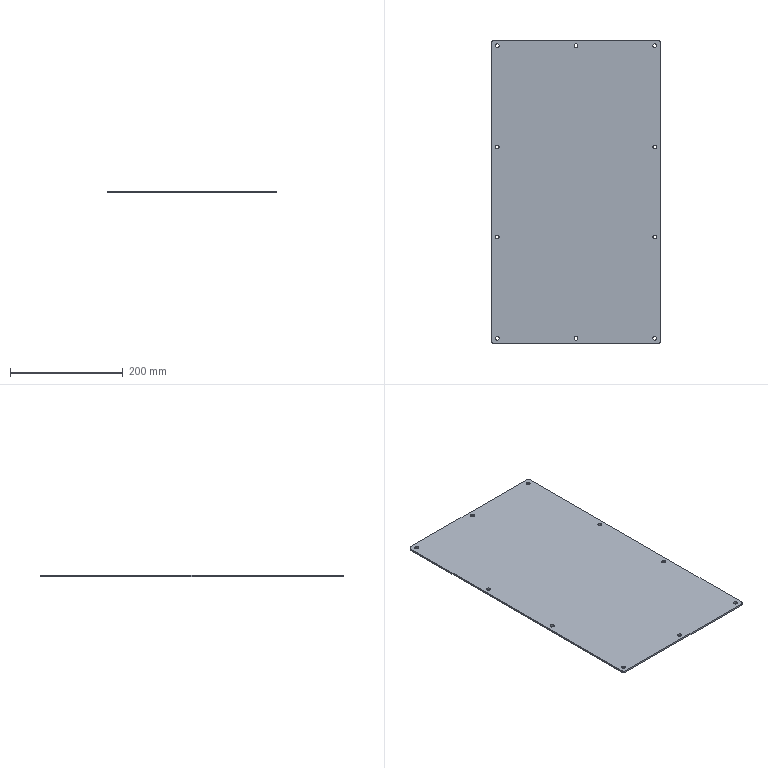Part | SolidWorks | features BaseBody 1 | 1 solid | 30 faces | box 300 x 540 x 3 mm | volume 484781 mm3 | cylinder 24 | plane 6 | commonest cylinder face diameters 7 x20 10 x4
STEP:
#1=CARTESIAN_POINT('',(136.5,-260.,0.));
#2=VERTEX_POINT('',#1);
#3=CARTESIAN_POINT('',(143.5,-260.,0.));
#4=VERTEX_POINT('',#3);
#5=CARTESIAN_POINT('',(140.,-260.,0.));
#6=DIRECTION('',(0.,0.,1.));
#7=DIRECTION('',(1.,0.,0.));
#8=AXIS2_PLACEMENT_3D('',#5,#6,#7);
#9=CIRCLE('',#8,3.5);
#10=EDGE_CURVE('',#2,#4,#9,.T.);
#11=ORIENTED_EDGE('',*,*,#10,.F.);
#12=CARTESIAN_POINT('',(136.5,-260.,3.));
#13=VERTEX_POINT('',#12);
#14=CARTESIAN_POINT('',(136.5,-260.,3.));
#15=DIRECTION('',(0.,0.,1.));
#16=VECTOR('',#15,1000.);
#17=LINE('',#14,#16);
#18=EDGE_CURVE('',#2,#13,#17,.T.);
#19=ORIENTED_EDGE('',*,*,#18,.T.);
#20=CARTESIAN_POINT('',(143.5,-260.,3.));
#21=VERTEX_POINT('',#20);
#22=CARTESIAN_POINT('',(140.,-260.,3.));
#23=DIRECTION('',(0.,0.,1.));
#24=DIRECTION('',(1.,0.,0.));
#25=AXIS2_PLACEMENT_3D('',#22,#23,#24);
#26=CIRCLE('',#25,3.5);
#27=EDGE_CURVE('',#13,#21,#26,.T.);
#28=ORIENTED_EDGE('',*,*,#27,.T.);
#29=CARTESIAN_POINT('',(143.5,-260.,3.));
#30=DIRECTION('',(0.,0.,1.));
#31=VECTOR('',#30,1000.);
#32=LINE('',#29,#31);
#33=EDGE_CURVE('',#4,#21,#32,.T.);
#34=ORIENTED_EDGE('',*,*,#33,.F.);
#35=EDGE_LOOP('',(#11,#19,#28,#34));
#36=FACE_OUTER_BOUND('',#35,.T.);
#37=CARTESIAN_POINT('',(140.,-260.,3.));
#38=DIRECTION('',(0.,0.,1.));
#39=DIRECTION('',(1.,0.,0.));
#40=AXIS2_PLACEMENT_3D('',#37,#38,#39);
#41=CYLINDRICAL_SURFACE('',#40,3.5);
#42=ADVANCED_FACE('',(#36),#41,.F.);
#43=CARTESIAN_POINT('',(-143.5,260.,0.));
#44=VERTEX_POINT('',#43);
#45=CARTESIAN_POINT('',(-136.5,260.,0.));
#46=VERTEX_POINT('',#45);
#47=CARTESIAN_POINT('',(-140.,260.,0.));
#48=DIRECTION('',(0.,0.,1.));
#49=DIRECTION('',(1.,0.,0.));
#50=AXIS2_PLACEMENT_3D('',#47,#48,#49);
#51=CIRCLE('',#50,3.5);
#52=EDGE_CURVE('',#44,#46,#51,.T.);
#53=ORIENTED_EDGE('',*,*,#52,.F.);
#54=CARTESIAN_POINT('',(-143.5,260.,3.));
#55=VERTEX_POINT('',#54);
#56=CARTESIAN_POINT('',(-143.5,260.,3.));
#57=DIRECTION('',(0.,0.,1.));
#58=VECTOR('',#57,1000.);
#59=LINE('',#56,#58);
#60=EDGE_CURVE('',#44,#55,#59,.T.);
#61=ORIENTED_EDGE('',*,*,#60,.T.);
#62=CARTESIAN_POINT('',(-136.5,260.,3.));
#63=VERTEX_POINT('',#62);
#64=CARTESIAN_POINT('',(-140.,260.,3.));
#65=DIRECTION('',(0.,0.,1.));
#66=DIRECTION('',(1.,0.,0.));
#67=AXIS2_PLACEMENT_3D('',#64,#65,#66);
#68=CIRCLE('',#67,3.5);
#69=EDGE_CURVE('',#55,#63,#68,.T.);
#70=ORIENTED_EDGE('',*,*,#69,.T.);
#71=CARTESIAN_POINT('',(-136.5,260.,3.));
#72=DIRECTION('',(0.,0.,1.));
#73=VECTOR('',#72,1000.);
#74=LINE('',#71,#73);
#75=EDGE_CURVE('',#46,#63,#74,.T.);
#76=ORIENTED_EDGE('',*,*,#75,.F.);
#77=EDGE_LOOP('',(#53,#61,#70,#76));
#78=FACE_OUTER_BOUND('',#77,.T.);
#79=CARTESIAN_POINT('',(-140.,260.,3.));
#80=DIRECTION('',(0.,0.,1.));
#81=DIRECTION('',(1.,0.,0.));
#82=AXIS2_PLACEMENT_3D('',#79,#80,#81);
#83=CYLINDRICAL_SURFACE('',#82,3.5);
#84=ADVANCED_FACE('',(#78),#83,.F.);
#85=CARTESIAN_POINT('',(-143.5,-260.,0.));
#86=VERTEX_POINT('',#85);
#87=CARTESIAN_POINT('',(-136.5,-260.,0.));
#88=VERTEX_POINT('',#87);
#89=CARTESIAN_POINT('',(-140.,-260.,0.));
#90=DIRECTION('',(0.,0.,1.));
#91=DIRECTION('',(1.,0.,0.));
#92=AXIS2_PLACEMENT_3D('',#89,#90,#91);
#93=CIRCLE('',#92,3.5);
#94=EDGE_CURVE('',#86,#88,#93,.T.);
#95=ORIENTED_EDGE('',*,*,#94,.F.);
#96=CARTESIAN_POINT('',(-143.5,-260.,3.));
#97=VERTEX_POINT('',#96);
#98=CARTESIAN_POINT('',(-143.5,-260.,3.));
#99=DIRECTION('',(0.,0.,1.));
#100=VECTOR('',#99,1000.);
#101=LINE('',#98,#100);
#102=EDGE_CURVE('',#86,#97,#101,.T.);
#103=ORIENTED_EDGE('',*,*,#102,.T.);
#104=CARTESIAN_POINT('',(-136.5,-260.,3.));
#105=VERTEX_POINT('',#104);
#106=CARTESIAN_POINT('',(-140.,-260.,3.));
#107=DIRECTION('',(0.,0.,1.));
#108=DIRECTION('',(1.,0.,0.));
#109=AXIS2_PLACEMENT_3D('',#106,#107,#108);
#110=CIRCLE('',#109,3.5);
#111=EDGE_CURVE('',#97,#105,#110,.T.);
#112=ORIENTED_EDGE('',*,*,#111,.T.);
#113=CARTESIAN_POINT('',(-136.5,-260.,3.));
#114=DIRECTION('',(0.,0.,1.));
#115=VECTOR('',#114,1000.);
#116=LINE('',#113,#115);
#117=EDGE_CURVE('',#88,#105,#116,.T.);
#118=ORIENTED_EDGE('',*,*,#117,.F.);
#119=EDGE_LOOP('',(#95,#103,#112,#118));
#120=FACE_OUTER_BOUND('',#119,.T.);
#121=CARTESIAN_POINT('',(-140.,-260.,3.));
#122=DIRECTION('',(0.,0.,1.));
#123=DIRECTION('',(1.,0.,0.));
#124=AXIS2_PLACEMENT_3D('',#121,#122,#123);
#125=CYLINDRICAL_SURFACE('',#124,3.5);
#126=ADVANCED_FACE('',(#120),#125,.F.);
#127=CARTESIAN_POINT('',(136.5,260.,0.));
#128=VERTEX_POINT('',#127);
#129=CARTESIAN_POINT('',(143.5,260.,0.));
#130=VERTEX_POINT('',#129);
#131=CARTESIAN_POINT('',(140.,260.,0.));
#132=DIRECTION('',(0.,0.,1.));
#133=DIRECTION('',(1.,0.,0.));
#134=AXIS2_PLACEMENT_3D('',#131,#132,#133);
#135=CIRCLE('',#134,3.5);
#136=EDGE_CURVE('',#128,#130,#135,.T.);
#137=ORIENTED_EDGE('',*,*,#136,.F.);
#138=CARTESIAN_POINT('',(136.5,260.,3.));
#139=VERTEX_POINT('',#138);
#140=CARTESIAN_POINT('',(136.5,260.,3.));
#141=DIRECTION('',(0.,0.,1.));
#142=VECTOR('',#141,1000.);
#143=LINE('',#140,#142);
#144=EDGE_CURVE('',#128,#139,#143,.T.);
#145=ORIENTED_EDGE('',*,*,#144,.T.);
#146=CARTESIAN_POINT('',(143.5,260.,3.));
#147=VERTEX_POINT('',#146);
#148=CARTESIAN_POINT('',(140.,260.,3.));
#149=DIRECTION('',(0.,0.,1.));
#150=DIRECTION('',(1.,0.,0.));
#151=AXIS2_PLACEMENT_3D('',#148,#149,#150);
#152=CIRCLE('',#151,3.5);
#153=EDGE_CURVE('',#139,#147,#152,.T.);
#154=ORIENTED_EDGE('',*,*,#153,.T.);
#155=CARTESIAN_POINT('',(143.5,260.,3.));
#156=DIRECTION('',(0.,0.,1.));
#157=VECTOR('',#156,1000.);
#158=LINE('',#155,#157);
#159=EDGE_CURVE('',#130,#147,#158,.T.);
#160=ORIENTED_EDGE('',*,*,#159,.F.);
#161=EDGE_LOOP('',(#137,#145,#154,#160));
#162=FACE_OUTER_BOUND('',#161,.T.);
#163=CARTESIAN_POINT('',(140.,260.,3.));
#164=DIRECTION('',(0.,0.,1.));
#165=DIRECTION('',(1.,0.,0.));
#166=AXIS2_PLACEMENT_3D('',#163,#164,#165);
#167=CYLINDRICAL_SURFACE('',#166,3.5);
#168=ADVANCED_FACE('',(#162),#167,.F.);
#169=CARTESIAN_POINT('',(-3.5,260.,0.));
#170=VERTEX_POINT('',#169);
#171=CARTESIAN_POINT('',(3.5,260.,0.));
#172=VERTEX_POINT('',#171);
#173=CARTESIAN_POINT('',(0.,260.,0.));
#174=DIRECTION('',(0.,0.,1.));
#175=DIRECTION('',(1.,0.,0.));
#176=AXIS2_PLACEMENT_3D('',#173,#174,#175);
#177=CIRCLE('',#176,3.5);
#178=EDGE_CURVE('',#170,#172,#177,.T.);
#179=ORIENTED_EDGE('',*,*,#178,.F.);
#180=CARTESIAN_POINT('',(-3.5,260.,3.));
#181=VERTEX_POINT('',#180);
#182=CARTESIAN_POINT('',(-3.5,260.,3.));
#183=DIRECTION('',(0.,0.,1.));
#184=VECTOR('',#183,1000.);
#185=LINE('',#182,#184);
#186=EDGE_CURVE('',#170,#181,#185,.T.);
#187=ORIENTED_EDGE('',*,*,#186,.T.);
#188=CARTESIAN_POINT('',(3.5,260.,3.));
#189=VERTEX_POINT('',#188);
#190=CARTESIAN_POINT('',(0.,260.,3.));
#191=DIRECTION('',(0.,0.,1.));
#192=DIRECTION('',(1.,0.,0.));
#193=AXIS2_PLACEMENT_3D('',#190,#191,#192);
#194=CIRCLE('',#193,3.5);
#195=EDGE_CURVE('',#181,#189,#194,.T.);
#196=ORIENTED_EDGE('',*,*,#195,.T.);
#197=CARTESIAN_POINT('',(3.5,260.,3.));
#198=DIRECTION('',(0.,0.,1.));
#199=VECTOR('',#198,1000.);
#200=LINE('',#197,#199);
#201=EDGE_CURVE('',#172,#189,#200,.T.);
#202=ORIENTED_EDGE('',*,*,#201,.F.);
#203=EDGE_LOOP('',(#179,#187,#196,#202));
#204=FACE_OUTER_BOUND('',#203,.T.);
#205=CARTESIAN_POINT('',(0.,260.,3.));
#206=DIRECTION('',(0.,0.,1.));
#207=DIRECTION('',(1.,0.,0.));
#208=AXIS2_PLACEMENT_3D('',#205,#206,#207);
#209=CYLINDRICAL_SURFACE('',#208,3.5);
#210=ADVANCED_FACE('',(#204),#209,.F.);
#211=CARTESIAN_POINT('',(-3.5,-260.,0.));
#212=VERTEX_POINT('',#211);
#213=CARTESIAN_POINT('',(3.5,-260.,0.));
#214=VERTEX_POINT('',#213);
#215=CARTESIAN_POINT('',(0.,-260.,0.));
#216=DIRECTION('',(0.,0.,1.));
#217=DIRECTION('',(1.,0.,0.));
#218=AXIS2_PLACEMENT_3D('',#215,#216,#217);
#219=CIRCLE('',#218,3.5);
#220=EDGE_CURVE('',#212,#214,#219,.T.);
#221=ORIENTED_EDGE('',*,*,#220,.F.);
#222=CARTESIAN_POINT('',(-3.5,-260.,3.));
#223=VERTEX_POINT('',#222);
#224=CARTESIAN_POINT('',(-3.5,-260.,3.));
#225=DIRECTION('',(0.,0.,1.));
#226=VECTOR('',#225,1000.);
#227=LINE('',#224,#226);
#228=EDGE_CURVE('',#212,#223,#227,.T.);
#229=ORIENTED_EDGE('',*,*,#228,.T.);
#230=CARTESIAN_POINT('',(3.5,-260.,3.));
#231=VERTEX_POINT('',#230);
#232=CARTESIAN_POINT('',(0.,-260.,3.));
#233=DIRECTION('',(0.,0.,1.));
#234=DIRECTION('',(1.,0.,0.));
#235=AXIS2_PLACEMENT_3D('',#232,#233,#234);
#236=CIRCLE('',#235,3.5);
#237=EDGE_CURVE('',#223,#231,#236,.T.);
#238=ORIENTED_EDGE('',*,*,#237,.T.);
#239=CARTESIAN_POINT('',(3.5,-260.,3.));
#240=DIRECTION('',(0.,0.,1.));
#241=VECTOR('',#240,1000.);
#242=LINE('',#239,#241);
#243=EDGE_CURVE('',#214,#231,#242,.T.);
#244=ORIENTED_EDGE('',*,*,#243,.F.);
#245=EDGE_LOOP('',(#221,#229,#238,#244));
#246=FACE_OUTER_BOUND('',#245,.T.);
#247=CARTESIAN_POINT('',(0.,-260.,3.));
#248=DIRECTION('',(0.,0.,1.));
#249=DIRECTION('',(1.,0.,0.));
#250=AXIS2_PLACEMENT_3D('',#247,#248,#249);
#251=CYLINDRICAL_SURFACE('',#250,3.5);
#252=ADVANCED_FACE('',(#246),#251,.F.);
#253=CARTESIAN_POINT('',(-143.5,-80.,0.));
#254=VERTEX_POINT('',#253);
#255=CARTESIAN_POINT('',(-136.5,-80.,0.));
#256=VERTEX_POINT('',#255);
#257=CARTESIAN_POINT('',(-140.,-80.,0.));
#258=DIRECTION('',(0.,0.,1.));
#259=DIRECTION('',(1.,0.,0.));
#260=AXIS2_PLACEMENT_3D('',#257,#258,#259);
#261=CIRCLE('',#260,3.5);
#262=EDGE_CURVE('',#254,#256,#261,.T.);
#263=ORIENTED_EDGE('',*,*,#262,.F.);
#264=CARTESIAN_POINT('',(-143.5,-80.,3.));
#265=VERTEX_POINT('',#264);
#266=CARTESIAN_POINT('',(-143.5,-80.,3.));
#267=DIRECTION('',(0.,0.,1.));
#268=VECTOR('',#267,1000.);
#269=LINE('',#266,#268);
#270=EDGE_CURVE('',#254,#265,#269,.T.);
#271=ORIENTED_EDGE('',*,*,#270,.T.);
#272=CARTESIAN_POINT('',(-136.5,-80.,3.));
#273=VERTEX_POINT('',#272);
#274=CARTESIAN_POINT('',(-140.,-80.,3.));
#275=DIRECTION('',(0.,0.,1.));
#276=DIRECTION('',(1.,0.,0.));
#277=AXIS2_PLACEMENT_3D('',#274,#275,#276);
#278=CIRCLE('',#277,3.5);
#279=EDGE_CURVE('',#265,#273,#278,.T.);
#280=ORIENTED_EDGE('',*,*,#279,.T.);
#281=CARTESIAN_POINT('',(-136.5,-80.,3.));
#282=DIRECTION('',(0.,0.,1.));
#283=VECTOR('',#282,1000.);
#284=LINE('',#281,#283);
#285=EDGE_CURVE('',#256,#273,#284,.T.);
#286=ORIENTED_EDGE('',*,*,#285,.F.);
#287=EDGE_LOOP('',(#263,#271,#280,#286));
#288=FACE_OUTER_BOUND('',#287,.T.);
#289=CARTESIAN_POINT('',(-140.,-80.,3.));
#290=DIRECTION('',(0.,0.,1.));
#291=DIRECTION('',(1.,0.,0.));
#292=AXIS2_PLACEMENT_3D('',#289,#290,#291);
#293=CYLINDRICAL_SURFACE('',#292,3.5);
#294=ADVANCED_FACE('',(#288),#293,.F.);
#295=CARTESIAN_POINT('',(-143.5,80.,0.));
#296=VERTEX_POINT('',#295);
#297=CARTESIAN_POINT('',(-136.5,80.,0.));
#298=VERTEX_POINT('',#297);
#299=CARTESIAN_POINT('',(-140.,80.,0.));
#300=DIRECTION('',(0.,0.,1.));
#301=DIRECTION('',(1.,0.,0.));
#302=AXIS2_PLACEMENT_3D('',#299,#300,#301);
#303=CIRCLE('',#302,3.5);
#304=EDGE_CURVE('',#296,#298,#303,.T.);
#305=ORIENTED_EDGE('',*,*,#304,.F.);
#306=CARTESIAN_POINT('',(-143.5,80.,3.));
#307=VERTEX_POINT('',#306);
#308=CARTESIAN_POINT('',(-143.5,80.,3.));
#309=DIRECTION('',(0.,0.,1.));
#310=VECTOR('',#309,1000.);
#311=LINE('',#308,#310);
#312=EDGE_CURVE('',#296,#307,#311,.T.);
#313=ORIENTED_EDGE('',*,*,#312,.T.);
#314=CARTESIAN_POINT('',(-136.5,80.,3.));
#315=VERTEX_POINT('',#314);
#316=CARTESIAN_POINT('',(-140.,80.,3.));
#317=DIRECTION('',(0.,0.,1.));
#318=DIRECTION('',(1.,0.,0.));
#319=AXIS2_PLACEMENT_3D('',#316,#317,#318);
#320=CIRCLE('',#319,3.5);
#321=EDGE_CURVE('',#307,#315,#320,.T.);
#322=ORIENTED_EDGE('',*,*,#321,.T.);
#323=CARTESIAN_POINT('',(-136.5,80.,3.));
#324=DIRECTION('',(0.,0.,1.));
#325=VECTOR('',#324,1000.);
#326=LINE('',#323,#325);
#327=EDGE_CURVE('',#298,#315,#326,.T.);
#328=ORIENTED_EDGE('',*,*,#327,.F.);
#329=EDGE_LOOP('',(#305,#313,#322,#328));
#330=FACE_OUTER_BOUND('',#329,.T.);
#331=CARTESIAN_POINT('',(-140.,80.,3.));
#332=DIRECTION('',(0.,0.,1.));
#333=DIRECTION('',(1.,0.,0.));
#334=AXIS2_PLACEMENT_3D('',#331,#332,#333);
#335=CYLINDRICAL_SURFACE('',#334,3.5);
#336=ADVANCED_FACE('',(#330),#335,.F.);
#337=CARTESIAN_POINT('',(136.5,80.,0.));
#338=VERTEX_POINT('',#337);
#339=CARTESIAN_POINT('',(143.5,80.,0.));
#340=VERTEX_POINT('',#339);
#341=CARTESIAN_POINT('',(140.,80.,0.));
#342=DIRECTION('',(0.,0.,1.));
#343=DIRECTION('',(1.,0.,0.));
#344=AXIS2_PLACEMENT_3D('',#341,#342,#343);
#345=CIRCLE('',#344,3.5);
#346=EDGE_CURVE('',#338,#340,#345,.T.);
#347=ORIENTED_EDGE('',*,*,#346,.F.);
#348=CARTESIAN_POINT('',(136.5,80.,3.));
#349=VERTEX_POINT('',#348);
#350=CARTESIAN_POINT('',(136.5,80.,3.));
#351=DIRECTION('',(0.,0.,1.));
#352=VECTOR('',#351,1000.);
#353=LINE('',#350,#352);
#354=EDGE_CURVE('',#338,#349,#353,.T.);
#355=ORIENTED_EDGE('',*,*,#354,.T.);
#356=CARTESIAN_POINT('',(143.5,80.,3.));
#357=VERTEX_POINT('',#356);
#358=CARTESIAN_POINT('',(140.,80.,3.));
#359=DIRECTION('',(0.,0.,1.));
#360=DIRECTION('',(1.,0.,0.));
#361=AXIS2_PLACEMENT_3D('',#358,#359,#360);
#362=CIRCLE('',#361,3.5);
#363=EDGE_CURVE('',#349,#357,#362,.T.);
#364=ORIENTED_EDGE('',*,*,#363,.T.);
#365=CARTESIAN_POINT('',(143.5,80.,3.));
#366=DIRECTION('',(0.,0.,1.));
#367=VECTOR('',#366,1000.);
#368=LINE('',#365,#367);
#369=EDGE_CURVE('',#340,#357,#368,.T.);
#370=ORIENTED_EDGE('',*,*,#369,.F.);
#371=EDGE_LOOP('',(#347,#355,#364,#370));
#372=FACE_OUTER_BOUND('',#371,.T.);
#373=CARTESIAN_POINT('',(140.,80.,3.));
#374=DIRECTION('',(0.,0.,1.));
#375=DIRECTION('',(1.,0.,0.));
#376=AXIS2_PLACEMENT_3D('',#373,#374,#375);
#377=CYLINDRICAL_SURFACE('',#376,3.5);
#378=ADVANCED_FACE('',(#372),#377,.F.);
#379=CARTESIAN_POINT('',(136.5,-80.,0.));
#380=VERTEX_POINT('',#379);
#381=CARTESIAN_POINT('',(143.5,-80.,0.));
#382=VERTEX_POINT('',#381);
#383=CARTESIAN_POINT('',(140.,-80.,0.));
#384=DIRECTION('',(0.,0.,1.));
#385=DIRECTION('',(1.,0.,0.));
#386=AXIS2_PLACEMENT_3D('',#383,#384,#385);
#387=CIRCLE('',#386,3.5);
#388=EDGE_CURVE('',#380,#382,#387,.T.);
#389=ORIENTED_EDGE('',*,*,#388,.F.);
#390=CARTESIAN_POINT('',(136.5,-80.,3.));
#391=VERTEX_POINT('',#390);
#392=CARTESIAN_POINT('',(136.5,-80.,3.));
#393=DIRECTION('',(0.,0.,1.));
#394=VECTOR('',#393,1000.);
#395=LINE('',#392,#394);
#396=EDGE_CURVE('',#380,#391,#395,.T.);
#397=ORIENTED_EDGE('',*,*,#396,.T.);
#398=CARTESIAN_POINT('',(143.5,-80.,3.));
#399=VERTEX_POINT('',#398);
#400=CARTESIAN_POINT('',(140.,-80.,3.));
#401=DIRECTION('',(0.,0.,1.));
#402=DIRECTION('',(1.,0.,0.));
#403=AXIS2_PLACEMENT_3D('',#400,#401,#402);
#404=CIRCLE('',#403,3.5);
#405=EDGE_CURVE('',#391,#399,#404,.T.);
#406=ORIENTED_EDGE('',*,*,#405,.T.);
#407=CARTESIAN_POINT('',(143.5,-80.,3.));
#408=DIRECTION('',(0.,0.,1.));
#409=VECTOR('',#408,1000.);
#410=LINE('',#407,#409);
#411=EDGE_CURVE('',#382,#399,#410,.T.);
#412=ORIENTED_EDGE('',*,*,#411,.F.);
#413=EDGE_LOOP('',(#389,#397,#406,#412));
#414=FACE_OUTER_BOUND('',#413,.T.);
#415=CARTESIAN_POINT('',(140.,-80.,3.));
#416=DIRECTION('',(0.,0.,1.));
#417=DIRECTION('',(1.,0.,0.));
#418=AXIS2_PLACEMENT_3D('',#415,#416,#417);
#419=CYLINDRICAL_SURFACE('',#418,3.5);
#420=ADVANCED_FACE('',(#414),#419,.F.);
#421=CARTESIAN_POINT('',(-150.,-265.,0.));
#422=VERTEX_POINT('',#421);
#423=CARTESIAN_POINT('',(-145.,-270.,0.));
#424=VERTEX_POINT('',#423);
#425=CARTESIAN_POINT('',(-145.,-265.,0.));
#426=DIRECTION('',(0.,0.,1.));
#427=DIRECTION('',(1.,0.,0.));
#428=AXIS2_PLACEMENT_3D('',#425,#426,#427);
#429=CIRCLE('',#428,5.);
#430=EDGE_CURVE('',#422,#424,#429,.T.);
#431=ORIENTED_EDGE('',*,*,#430,.T.);
#432=CARTESIAN_POINT('',(-145.,-270.,3.));
#433=VERTEX_POINT('',#432);
#434=CARTESIAN_POINT('',(-145.,-270.,3.));
#435=DIRECTION('',(0.,0.,-1.));
#436=VECTOR('',#435,1000.);
#437=LINE('',#434,#436);
#438=EDGE_CURVE('',#433,#424,#437,.T.);
#439=ORIENTED_EDGE('',*,*,#438,.F.);
#440=CARTESIAN_POINT('',(-150.,-265.,3.));
#441=VERTEX_POINT('',#440);
#442=CARTESIAN_POINT('',(-145.,-265.,3.));
#443=DIRECTION('',(0.,0.,1.));
#444=DIRECTION('',(1.,0.,0.));
#445=AXIS2_PLACEMENT_3D('',#442,#443,#444);
#446=CIRCLE('',#445,5.);
#447=EDGE_CURVE('',#441,#433,#446,.T.);
#448=ORIENTED_EDGE('',*,*,#447,.F.);
#449=CARTESIAN_POINT('',(-150.,-265.,3.));
#450=DIRECTION('',(0.,0.,-1.));
#451=VECTOR('',#450,1000.);
#452=LINE('',#449,#451);
#453=EDGE_CURVE('',#441,#422,#452,.T.);
#454=ORIENTED_EDGE('',*,*,#453,.T.);
#455=EDGE_LOOP('',(#431,#439,#448,#454));
#456=FACE_OUTER_BOUND('',#455,.T.);
#457=CARTESIAN_POINT('',(-145.,-265.,3.));
#458=DIRECTION('',(0.,0.,-1.));
#459=DIRECTION('',(-1.,0.,0.));
#460=AXIS2_PLACEMENT_3D('',#457,#458,#459);
#461=CYLINDRICAL_SURFACE('',#460,5.);
#462=ADVANCED_FACE('',(#456),#461,.T.);
#463=CARTESIAN_POINT('',(145.,-270.,0.));
#464=VERTEX_POINT('',#463);
#465=CARTESIAN_POINT('',(-145.,-270.,0.));
#466=DIRECTION('',(1.,0.,0.));
#467=VECTOR('',#466,1000.);
#468=LINE('',#465,#467);
#469=EDGE_CURVE('',#424,#464,#468,.T.);
#470=ORIENTED_EDGE('',*,*,#469,.T.);
#471=CARTESIAN_POINT('',(145.,-270.,3.));
#472=VERTEX_POINT('',#471);
#473=CARTESIAN_POINT('',(145.,-270.,3.));
#474=DIRECTION('',(0.,0.,-1.));
#475=VECTOR('',#474,1000.);
#476=LINE('',#473,#475);
#477=EDGE_CURVE('',#472,#464,#476,.T.);
#478=ORIENTED_EDGE('',*,*,#477,.F.);
#479=CARTESIAN_POINT('',(-145.,-270.,3.));
#480=DIRECTION('',(1.,0.,0.));
#481=VECTOR('',#480,1000.);
#482=LINE('',#479,#481);
#483=EDGE_CURVE('',#433,#472,#482,.T.);
#484=ORIENTED_EDGE('',*,*,#483,.F.);
#485=ORIENTED_EDGE('',*,*,#438,.T.);
#486=EDGE_LOOP('',(#470,#478,#484,#485));
#487=FACE_OUTER_BOUND('',#486,.T.);
#488=CARTESIAN_POINT('',(-145.,-270.,3.));
#489=DIRECTION('',(0.,1.,0.));
#490=DIRECTION('',(0.,0.,1.));
#491=AXIS2_PLACEMENT_3D('',#488,#489,#490);
#492=PLANE('',#491);
#493=ADVANCED_FACE('',(#487),#492,.F.);
#494=CARTESIAN_POINT('',(150.,-265.,0.));
#495=VERTEX_POINT('',#494);
#496=CARTESIAN_POINT('',(145.,-265.,0.));
#497=DIRECTION('',(0.,0.,1.));
#498=DIRECTION('',(1.,0.,0.));
#499=AXIS2_PLACEMENT_3D('',#496,#497,#498);
#500=CIRCLE('',#499,5.);
#501=EDGE_CURVE('',#464,#495,#500,.T.);
#502=ORIENTED_EDGE('',*,*,#501,.T.);
#503=CARTESIAN_POINT('',(150.,-265.,3.));
#504=VERTEX_POINT('',#503);
#505=CARTESIAN_POINT('',(150.,-265.,3.));
#506=DIRECTION('',(0.,0.,-1.));
#507=VECTOR('',#506,1000.);
#508=LINE('',#505,#507);
#509=EDGE_CURVE('',#504,#495,#508,.T.);
#510=ORIENTED_EDGE('',*,*,#509,.F.);
#511=CARTESIAN_POINT('',(145.,-265.,3.));
#512=DIRECTION('',(0.,0.,1.));
#513=DIRECTION('',(1.,0.,0.));
#514=AXIS2_PLACEMENT_3D('',#511,#512,#513);
#515=CIRCLE('',#514,5.);
#516=EDGE_CURVE('',#472,#504,#515,.T.);
#517=ORIENTED_EDGE('',*,*,#516,.F.);
#518=ORIENTED_EDGE('',*,*,#477,.T.);
#519=EDGE_LOOP('',(#502,#510,#517,#518));
#520=FACE_OUTER_BOUND('',#519,.T.);
#521=CARTESIAN_POINT('',(145.,-265.,3.));
#522=DIRECTION('',(0.,0.,-1.));
#523=DIRECTION('',(-1.,0.,0.));
#524=AXIS2_PLACEMENT_3D('',#521,#522,#523);
#525=CYLINDRICAL_SURFACE('',#524,5.);
#526=ADVANCED_FACE('',(#520),#525,.T.);
#527=CARTESIAN_POINT('',(150.,265.,0.));
#528=VERTEX_POINT('',#527);
#529=CARTESIAN_POINT('',(150.,265.,0.));
#530=DIRECTION('',(0.,1.,0.));
#531=VECTOR('',#530,1000.);
#532=LINE('',#529,#531);
#533=EDGE_CURVE('',#495,#528,#532,.T.);
#534=ORIENTED_EDGE('',*,*,#533,.T.);
#535=CARTESIAN_POINT('',(150.,265.,3.));
#536=VERTEX_POINT('',#535);
#537=CARTESIAN_POINT('',(150.,265.,3.));
#538=DIRECTION('',(0.,0.,-1.));
#539=VECTOR('',#538,1000.);
#540=LINE('',#537,#539);
#541=EDGE_CURVE('',#536,#528,#540,.T.);
#542=ORIENTED_EDGE('',*,*,#541,.F.);
#543=CARTESIAN_POINT('',(150.,265.,3.));
#544=DIRECTION('',(0.,1.,0.));
#545=VECTOR('',#544,1000.);
#546=LINE('',#543,#545);
#547=EDGE_CURVE('',#504,#536,#546,.T.);
#548=ORIENTED_EDGE('',*,*,#547,.F.);
#549=ORIENTED_EDGE('',*,*,#509,.T.);
#550=EDGE_LOOP('',(#534,#542,#548,#549));
#551=FACE_OUTER_BOUND('',#550,.T.);
#552=CARTESIAN_POINT('',(150.,265.,3.));
#553=DIRECTION('',(-1.,0.,0.));
#554=DIRECTION('',(0.,-1.,0.));
#555=AXIS2_PLACEMENT_3D('',#552,#553,#554);
#556=PLANE('',#555);
#557=ADVANCED_FACE('',(#551),#556,.F.);
#558=CARTESIAN_POINT('',(145.,270.,0.));
#559=VERTEX_POINT('',#558);
#560=CARTESIAN_POINT('',(145.,265.,0.));
#561=DIRECTION('',(0.,0.,1.));
#562=DIRECTION('',(-1.,0.,0.));
#563=AXIS2_PLACEMENT_3D('',#560,#561,#562);
#564=CIRCLE('',#563,5.);
#565=EDGE_CURVE('',#528,#559,#564,.T.);
#566=ORIENTED_EDGE('',*,*,#565,.T.);
#567=CARTESIAN_POINT('',(145.,270.,3.));
#568=VERTEX_POINT('',#567);
#569=CARTESIAN_POINT('',(145.,270.,3.));
#570=DIRECTION('',(0.,0.,-1.));
#571=VECTOR('',#570,1000.);
#572=LINE('',#569,#571);
#573=EDGE_CURVE('',#568,#559,#572,.T.);
#574=ORIENTED_EDGE('',*,*,#573,.F.);
#575=CARTESIAN_POINT('',(145.,265.,3.));
#576=DIRECTION('',(0.,0.,1.));
#577=DIRECTION('',(-1.,0.,0.));
#578=AXIS2_PLACEMENT_3D('',#575,#576,#577);
#579=CIRCLE('',#578,5.);
#580=EDGE_CURVE('',#536,#568,#579,.T.);
#581=ORIENTED_EDGE('',*,*,#580,.F.);
#582=ORIENTED_EDGE('',*,*,#541,.T.);
#583=EDGE_LOOP('',(#566,#574,#581,#582));
#584=FACE_OUTER_BOUND('',#583,.T.);
#585=CARTESIAN_POINT('',(145.,265.,3.));
#586=DIRECTION('',(0.,0.,-1.));
#587=DIRECTION('',(-1.,0.,0.));
#588=AXIS2_PLACEMENT_3D('',#585,#586,#587);
#589=CYLINDRICAL_SURFACE('',#588,5.);
#590=ADVANCED_FACE('',(#584),#589,.T.);
#591=CARTESIAN_POINT('',(-145.,270.,0.));
#592=VERTEX_POINT('',#591);
#593=CARTESIAN_POINT('',(-145.,270.,0.));
#594=DIRECTION('',(-1.,0.,0.));
#595=VECTOR('',#594,1000.);
#596=LINE('',#593,#595);
#597=EDGE_CURVE('',#559,#592,#596,.T.);
#598=ORIENTED_EDGE('',*,*,#597,.T.);
#599=CARTESIAN_POINT('',(-145.,270.,3.));
#600=VERTEX_POINT('',#599);
#601=CARTESIAN_POINT('',(-145.,270.,3.));
#602=DIRECTION('',(0.,0.,-1.));
#603=VECTOR('',#602,1000.);
#604=LINE('',#601,#603);
#605=EDGE_CURVE('',#600,#592,#604,.T.);
#606=ORIENTED_EDGE('',*,*,#605,.F.);
#607=CARTESIAN_POINT('',(-145.,270.,3.));
#608=DIRECTION('',(-1.,0.,0.));
#609=VECTOR('',#608,1000.);
#610=LINE('',#607,#609);
#611=EDGE_CURVE('',#568,#600,#610,.T.);
#612=ORIENTED_EDGE('',*,*,#611,.F.);
#613=ORIENTED_EDGE('',*,*,#573,.T.);
#614=EDGE_LOOP('',(#598,#606,#612,#613));
#615=FACE_OUTER_BOUND('',#614,.T.);
#616=CARTESIAN_POINT('',(-145.,270.,3.));
#617=DIRECTION('',(0.,-1.,0.));
#618=DIRECTION('',(0.,0.,-1.));
#619=AXIS2_PLACEMENT_3D('',#616,#617,#618);
#620=PLANE('',#619);
#621=ADVANCED_FACE('',(#615),#620,.F.);
#622=CARTESIAN_POINT('',(-150.,265.,0.));
#623=VERTEX_POINT('',#622);
#624=CARTESIAN_POINT('',(-145.,265.,0.));
#625=DIRECTION('',(0.,0.,1.));
#626=DIRECTION('',(1.,0.,0.));
#627=AXIS2_PLACEMENT_3D('',#624,#625,#626);
#628=CIRCLE('',#627,5.);
#629=EDGE_CURVE('',#592,#623,#628,.T.);
#630=ORIENTED_EDGE('',*,*,#629,.T.);
#631=CARTESIAN_POINT('',(-150.,265.,3.));
#632=VERTEX_POINT('',#631);
#633=CARTESIAN_POINT('',(-150.,265.,3.));
#634=DIRECTION('',(0.,0.,-1.));
#635=VECTOR('',#634,1000.);
#636=LINE('',#633,#635);
#637=EDGE_CURVE('',#632,#623,#636,.T.);
#638=ORIENTED_EDGE('',*,*,#637,.F.);
#639=CARTESIAN_POINT('',(-145.,265.,3.));
#640=DIRECTION('',(0.,0.,1.));
#641=DIRECTION('',(1.,0.,0.));
#642=AXIS2_PLACEMENT_3D('',#639,#640,#641);
#643=CIRCLE('',#642,5.);
#644=EDGE_CURVE('',#600,#632,#643,.T.);
#645=ORIENTED_EDGE('',*,*,#644,.F.);
#646=ORIENTED_EDGE('',*,*,#605,.T.);
#647=EDGE_LOOP('',(#630,#638,#645,#646));
#648=FACE_OUTER_BOUND('',#647,.T.);
#649=CARTESIAN_POINT('',(-145.,265.,3.));
#650=DIRECTION('',(0.,0.,-1.));
#651=DIRECTION('',(-1.,0.,0.));
#652=AXIS2_PLACEMENT_3D('',#649,#650,#651);
#653=CYLINDRICAL_SURFACE('',#652,5.);
#654=ADVANCED_FACE('',(#648),#653,.T.);
#655=CARTESIAN_POINT('',(-150.,265.,0.));
#656=DIRECTION('',(0.,-1.,0.));
#657=VECTOR('',#656,1000.);
#658=LINE('',#655,#657);
#659=EDGE_CURVE('',#623,#422,#658,.T.);
#660=ORIENTED_EDGE('',*,*,#659,.T.);
#661=ORIENTED_EDGE('',*,*,#453,.F.);
#662=CARTESIAN_POINT('',(-150.,265.,3.));
#663=DIRECTION('',(0.,-1.,0.));
#664=VECTOR('',#663,1000.);
#665=LINE('',#662,#664);
#666=EDGE_CURVE('',#632,#441,#665,.T.);
#667=ORIENTED_EDGE('',*,*,#666,.F.);
#668=ORIENTED_EDGE('',*,*,#637,.T.);
#669=EDGE_LOOP('',(#660,#661,#667,#668));
#670=FACE_OUTER_BOUND('',#669,.T.);
#671=CARTESIAN_POINT('',(-150.,265.,3.));
#672=DIRECTION('',(1.,0.,0.));
#673=DIRECTION('',(0.,0.,-1.));
#674=AXIS2_PLACEMENT_3D('',#671,#672,#673);
#675=PLANE('',#674);
#676=ADVANCED_FACE('',(#670),#675,.F.);
#677=CARTESIAN_POINT('',(140.,-260.,3.));
#678=DIRECTION('',(0.,0.,1.));
#679=DIRECTION('',(1.,0.,0.));
#680=AXIS2_PLACEMENT_3D('',#677,#678,#679);
#681=CIRCLE('',#680,3.5);
#682=EDGE_CURVE('',#21,#13,#681,.T.);
#683=ORIENTED_EDGE('',*,*,#682,.F.);
#684=ORIENTED_EDGE('',*,*,#27,.F.);
#685=EDGE_LOOP('',(#683,#684));
#686=FACE_BOUND('',#685,.T.);
#687=CARTESIAN_POINT('',(-140.,260.,3.));
#688=DIRECTION('',(0.,0.,1.));
#689=DIRECTION('',(1.,0.,0.));
#690=AXIS2_PLACEMENT_3D('',#687,#688,#689);
#691=CIRCLE('',#690,3.5);
#692=EDGE_CURVE('',#63,#55,#691,.T.);
#693=ORIENTED_EDGE('',*,*,#692,.F.);
#694=ORIENTED_EDGE('',*,*,#69,.F.);
#695=EDGE_LOOP('',(#693,#694));
#696=FACE_BOUND('',#695,.T.);
#697=CARTESIAN_POINT('',(-140.,-260.,3.));
#698=DIRECTION('',(0.,0.,1.));
#699=DIRECTION('',(1.,0.,0.));
#700=AXIS2_PLACEMENT_3D('',#697,#698,#699);
#701=CIRCLE('',#700,3.5);
#702=EDGE_CURVE('',#105,#97,#701,.T.);
#703=ORIENTED_EDGE('',*,*,#702,.F.);
#704=ORIENTED_EDGE('',*,*,#111,.F.);
#705=EDGE_LOOP('',(#703,#704));
#706=FACE_BOUND('',#705,.T.);
#707=CARTESIAN_POINT('',(140.,260.,3.));
#708=DIRECTION('',(0.,0.,1.));
#709=DIRECTION('',(1.,0.,0.));
#710=AXIS2_PLACEMENT_3D('',#707,#708,#709);
#711=CIRCLE('',#710,3.5);
#712=EDGE_CURVE('',#147,#139,#711,.T.);
#713=ORIENTED_EDGE('',*,*,#712,.F.);
#714=ORIENTED_EDGE('',*,*,#153,.F.);
#715=EDGE_LOOP('',(#713,#714));
#716=FACE_BOUND('',#715,.T.);
#717=CARTESIAN_POINT('',(0.,260.,3.));
#718=DIRECTION('',(0.,0.,1.));
#719=DIRECTION('',(1.,0.,0.));
#720=AXIS2_PLACEMENT_3D('',#717,#718,#719);
#721=CIRCLE('',#720,3.5);
#722=EDGE_CURVE('',#189,#181,#721,.T.);
#723=ORIENTED_EDGE('',*,*,#722,.F.);
#724=ORIENTED_EDGE('',*,*,#195,.F.);
#725=EDGE_LOOP('',(#723,#724));
#726=FACE_BOUND('',#725,.T.);
#727=CARTESIAN_POINT('',(0.,-260.,3.));
#728=DIRECTION('',(0.,0.,1.));
#729=DIRECTION('',(1.,0.,0.));
#730=AXIS2_PLACEMENT_3D('',#727,#728,#729);
#731=CIRCLE('',#730,3.5);
#732=EDGE_CURVE('',#231,#223,#731,.T.);
#733=ORIENTED_EDGE('',*,*,#732,.F.);
#734=ORIENTED_EDGE('',*,*,#237,.F.);
#735=EDGE_LOOP('',(#733,#734));
#736=FACE_BOUND('',#735,.T.);
#737=CARTESIAN_POINT('',(-140.,-80.,3.));
#738=DIRECTION('',(0.,0.,1.));
#739=DIRECTION('',(1.,0.,0.));
#740=AXIS2_PLACEMENT_3D('',#737,#738,#739);
#741=CIRCLE('',#740,3.5);
#742=EDGE_CURVE('',#273,#265,#741,.T.);
#743=ORIENTED_EDGE('',*,*,#742,.F.);
#744=ORIENTED_EDGE('',*,*,#279,.F.);
#745=EDGE_LOOP('',(#743,#744));
#746=FACE_BOUND('',#745,.T.);
#747=CARTESIAN_POINT('',(-140.,80.,3.));
#748=DIRECTION('',(0.,0.,1.));
#749=DIRECTION('',(1.,0.,0.));
#750=AXIS2_PLACEMENT_3D('',#747,#748,#749);
#751=CIRCLE('',#750,3.5);
#752=EDGE_CURVE('',#315,#307,#751,.T.);
#753=ORIENTED_EDGE('',*,*,#752,.F.);
#754=ORIENTED_EDGE('',*,*,#321,.F.);
#755=EDGE_LOOP('',(#753,#754));
#756=FACE_BOUND('',#755,.T.);
#757=CARTESIAN_POINT('',(140.,80.,3.));
#758=DIRECTION('',(0.,0.,1.));
#759=DIRECTION('',(1.,0.,0.));
#760=AXIS2_PLACEMENT_3D('',#757,#758,#759);
#761=CIRCLE('',#760,3.5);
#762=EDGE_CURVE('',#357,#349,#761,.T.);
#763=ORIENTED_EDGE('',*,*,#762,.F.);
#764=ORIENTED_EDGE('',*,*,#363,.F.);
#765=EDGE_LOOP('',(#763,#764));
#766=FACE_BOUND('',#765,.T.);
#767=CARTESIAN_POINT('',(140.,-80.,3.));
#768=DIRECTION('',(0.,0.,1.));
#769=DIRECTION('',(1.,0.,0.));
#770=AXIS2_PLACEMENT_3D('',#767,#768,#769);
#771=CIRCLE('',#770,3.5);
#772=EDGE_CURVE('',#399,#391,#771,.T.);
#773=ORIENTED_EDGE('',*,*,#772,.F.);
#774=ORIENTED_EDGE('',*,*,#405,.F.);
#775=EDGE_LOOP('',(#773,#774));
#776=FACE_BOUND('',#775,.T.);
#777=ORIENTED_EDGE('',*,*,#447,.T.);
#778=ORIENTED_EDGE('',*,*,#483,.T.);
#779=ORIENTED_EDGE('',*,*,#516,.T.);
#780=ORIENTED_EDGE('',*,*,#547,.T.);
#781=ORIENTED_EDGE('',*,*,#580,.T.);
#782=ORIENTED_EDGE('',*,*,#611,.T.);
#783=ORIENTED_EDGE('',*,*,#644,.T.);
#784=ORIENTED_EDGE('',*,*,#666,.T.);
#785=EDGE_LOOP('',(#777,#778,#779,#780,#781,#782,#783,#784));
#786=FACE_OUTER_BOUND('',#785,.T.);
#787=CARTESIAN_POINT('',(-145.,-265.,3.));
#788=DIRECTION('',(0.,0.,1.));
#789=DIRECTION('',(1.,0.,0.));
#790=AXIS2_PLACEMENT_3D('',#787,#788,#789);
#791=PLANE('',#790);
#792=ADVANCED_FACE('',(#686,#696,#706,#716,#726,#736,#746,#756,#766,#776,#786),#791,.T.);
#793=CARTESIAN_POINT('',(140.,-260.,0.));
#794=DIRECTION('',(0.,0.,1.));
#795=DIRECTION('',(1.,0.,0.));
#796=AXIS2_PLACEMENT_3D('',#793,#794,#795);
#797=CIRCLE('',#796,3.5);
#798=EDGE_CURVE('',#4,#2,#797,.T.);
#799=ORIENTED_EDGE('',*,*,#798,.T.);
#800=ORIENTED_EDGE('',*,*,#10,.T.);
#801=EDGE_LOOP('',(#799,#800));
#802=FACE_BOUND('',#801,.T.);
#803=CARTESIAN_POINT('',(-140.,260.,0.));
#804=DIRECTION('',(0.,0.,1.));
#805=DIRECTION('',(1.,0.,0.));
#806=AXIS2_PLACEMENT_3D('',#803,#804,#805);
#807=CIRCLE('',#806,3.5);
#808=EDGE_CURVE('',#46,#44,#807,.T.);
#809=ORIENTED_EDGE('',*,*,#808,.T.);
#810=ORIENTED_EDGE('',*,*,#52,.T.);
#811=EDGE_LOOP('',(#809,#810));
#812=FACE_BOUND('',#811,.T.);
#813=CARTESIAN_POINT('',(-140.,-260.,0.));
#814=DIRECTION('',(0.,0.,1.));
#815=DIRECTION('',(1.,0.,0.));
#816=AXIS2_PLACEMENT_3D('',#813,#814,#815);
#817=CIRCLE('',#816,3.5);
#818=EDGE_CURVE('',#88,#86,#817,.T.);
#819=ORIENTED_EDGE('',*,*,#818,.T.);
#820=ORIENTED_EDGE('',*,*,#94,.T.);
#821=EDGE_LOOP('',(#819,#820));
#822=FACE_BOUND('',#821,.T.);
#823=CARTESIAN_POINT('',(140.,260.,0.));
#824=DIRECTION('',(0.,0.,1.));
#825=DIRECTION('',(1.,0.,0.));
#826=AXIS2_PLACEMENT_3D('',#823,#824,#825);
#827=CIRCLE('',#826,3.5);
#828=EDGE_CURVE('',#130,#128,#827,.T.);
#829=ORIENTED_EDGE('',*,*,#828,.T.);
#830=ORIENTED_EDGE('',*,*,#136,.T.);
#831=EDGE_LOOP('',(#829,#830));
#832=FACE_BOUND('',#831,.T.);
#833=CARTESIAN_POINT('',(0.,260.,0.));
#834=DIRECTION('',(0.,0.,1.));
#835=DIRECTION('',(1.,0.,0.));
#836=AXIS2_PLACEMENT_3D('',#833,#834,#835);
#837=CIRCLE('',#836,3.5);
#838=EDGE_CURVE('',#172,#170,#837,.T.);
#839=ORIENTED_EDGE('',*,*,#838,.T.);
#840=ORIENTED_EDGE('',*,*,#178,.T.);
#841=EDGE_LOOP('',(#839,#840));
#842=FACE_BOUND('',#841,.T.);
#843=CARTESIAN_POINT('',(0.,-260.,0.));
#844=DIRECTION('',(0.,0.,1.));
#845=DIRECTION('',(1.,0.,0.));
#846=AXIS2_PLACEMENT_3D('',#843,#844,#845);
#847=CIRCLE('',#846,3.5);
#848=EDGE_CURVE('',#214,#212,#847,.T.);
#849=ORIENTED_EDGE('',*,*,#848,.T.);
#850=ORIENTED_EDGE('',*,*,#220,.T.);
#851=EDGE_LOOP('',(#849,#850));
#852=FACE_BOUND('',#851,.T.);
#853=CARTESIAN_POINT('',(-140.,-80.,0.));
#854=DIRECTION('',(0.,0.,1.));
#855=DIRECTION('',(1.,0.,0.));
#856=AXIS2_PLACEMENT_3D('',#853,#854,#855);
#857=CIRCLE('',#856,3.5);
#858=EDGE_CURVE('',#256,#254,#857,.T.);
#859=ORIENTED_EDGE('',*,*,#858,.T.);
#860=ORIENTED_EDGE('',*,*,#262,.T.);
#861=EDGE_LOOP('',(#859,#860));
#862=FACE_BOUND('',#861,.T.);
#863=CARTESIAN_POINT('',(-140.,80.,0.));
#864=DIRECTION('',(0.,0.,1.));
#865=DIRECTION('',(1.,0.,0.));
#866=AXIS2_PLACEMENT_3D('',#863,#864,#865);
#867=CIRCLE('',#866,3.5);
#868=EDGE_CURVE('',#298,#296,#867,.T.);
#869=ORIENTED_EDGE('',*,*,#868,.T.);
#870=ORIENTED_EDGE('',*,*,#304,.T.);
#871=EDGE_LOOP('',(#869,#870));
#872=FACE_BOUND('',#871,.T.);
#873=CARTESIAN_POINT('',(140.,80.,0.));
#874=DIRECTION('',(0.,0.,1.));
#875=DIRECTION('',(1.,0.,0.));
#876=AXIS2_PLACEMENT_3D('',#873,#874,#875);
#877=CIRCLE('',#876,3.5);
#878=EDGE_CURVE('',#340,#338,#877,.T.);
#879=ORIENTED_EDGE('',*,*,#878,.T.);
#880=ORIENTED_EDGE('',*,*,#346,.T.);
#881=EDGE_LOOP('',(#879,#880));
#882=FACE_BOUND('',#881,.T.);
#883=CARTESIAN_POINT('',(140.,-80.,0.));
#884=DIRECTION('',(0.,0.,1.));
#885=DIRECTION('',(1.,0.,0.));
#886=AXIS2_PLACEMENT_3D('',#883,#884,#885);
#887=CIRCLE('',#886,3.5);
#888=EDGE_CURVE('',#382,#380,#887,.T.);
#889=ORIENTED_EDGE('',*,*,#888,.T.);
#890=ORIENTED_EDGE('',*,*,#388,.T.);
#891=EDGE_LOOP('',(#889,#890));
#892=FACE_BOUND('',#891,.T.);
#893=ORIENTED_EDGE('',*,*,#430,.F.);
#894=ORIENTED_EDGE('',*,*,#659,.F.);
#895=ORIENTED_EDGE('',*,*,#629,.F.);
#896=ORIENTED_EDGE('',*,*,#597,.F.);
#897=ORIENTED_EDGE('',*,*,#565,.F.);
#898=ORIENTED_EDGE('',*,*,#533,.F.);
#899=ORIENTED_EDGE('',*,*,#501,.F.);
#900=ORIENTED_EDGE('',*,*,#469,.F.);
#901=EDGE_LOOP('',(#893,#894,#895,#896,#897,#898,#899,#900));
#902=FACE_OUTER_BOUND('',#901,.T.);
#903=CARTESIAN_POINT('',(-145.,-265.,0.));
#904=DIRECTION('',(0.,0.,1.));
#905=DIRECTION('',(1.,0.,0.));
#906=AXIS2_PLACEMENT_3D('',#903,#904,#905);
#907=PLANE('',#906);
#908=ADVANCED_FACE('',(#802,#812,#822,#832,#842,#852,#862,#872,#882,#892,#902),#907,.F.);
#909=ORIENTED_EDGE('',*,*,#396,.F.);
#910=ORIENTED_EDGE('',*,*,#888,.F.);
#911=ORIENTED_EDGE('',*,*,#411,.T.);
#912=ORIENTED_EDGE('',*,*,#772,.T.);
#913=EDGE_LOOP('',(#909,#910,#911,#912));
#914=FACE_OUTER_BOUND('',#913,.T.);
#915=CARTESIAN_POINT('',(140.,-80.,3.));
#916=DIRECTION('',(0.,0.,1.));
#917=DIRECTION('',(1.,0.,0.));
#918=AXIS2_PLACEMENT_3D('',#915,#916,#917);
#919=CYLINDRICAL_SURFACE('',#918,3.5);
#920=ADVANCED_FACE('',(#914),#919,.F.);
#921=ORIENTED_EDGE('',*,*,#354,.F.);
#922=ORIENTED_EDGE('',*,*,#878,.F.);
#923=ORIENTED_EDGE('',*,*,#369,.T.);
#924=ORIENTED_EDGE('',*,*,#762,.T.);
#925=EDGE_LOOP('',(#921,#922,#923,#924));
#926=FACE_OUTER_BOUND('',#925,.T.);
#927=CARTESIAN_POINT('',(140.,80.,3.));
#928=DIRECTION('',(0.,0.,1.));
#929=DIRECTION('',(1.,0.,0.));
#930=AXIS2_PLACEMENT_3D('',#927,#928,#929);
#931=CYLINDRICAL_SURFACE('',#930,3.5);
#932=ADVANCED_FACE('',(#926),#931,.F.);
#933=ORIENTED_EDGE('',*,*,#312,.F.);
#934=ORIENTED_EDGE('',*,*,#868,.F.);
#935=ORIENTED_EDGE('',*,*,#327,.T.);
#936=ORIENTED_EDGE('',*,*,#752,.T.);
#937=EDGE_LOOP('',(#933,#934,#935,#936));
#938=FACE_OUTER_BOUND('',#937,.T.);
#939=CARTESIAN_POINT('',(-140.,80.,3.));
#940=DIRECTION('',(0.,0.,1.));
#941=DIRECTION('',(1.,0.,0.));
#942=AXIS2_PLACEMENT_3D('',#939,#940,#941);
#943=CYLINDRICAL_SURFACE('',#942,3.5);
#944=ADVANCED_FACE('',(#938),#943,.F.);
#945=ORIENTED_EDGE('',*,*,#270,.F.);
#946=ORIENTED_EDGE('',*,*,#858,.F.);
#947=ORIENTED_EDGE('',*,*,#285,.T.);
#948=ORIENTED_EDGE('',*,*,#742,.T.);
#949=EDGE_LOOP('',(#945,#946,#947,#948));
#950=FACE_OUTER_BOUND('',#949,.T.);
#951=CARTESIAN_POINT('',(-140.,-80.,3.));
#952=DIRECTION('',(0.,0.,1.));
#953=DIRECTION('',(1.,0.,0.));
#954=AXIS2_PLACEMENT_3D('',#951,#952,#953);
#955=CYLINDRICAL_SURFACE('',#954,3.5);
#956=ADVANCED_FACE('',(#950),#955,.F.);
#957=ORIENTED_EDGE('',*,*,#228,.F.);
#958=ORIENTED_EDGE('',*,*,#848,.F.);
#959=ORIENTED_EDGE('',*,*,#243,.T.);
#960=ORIENTED_EDGE('',*,*,#732,.T.);
#961=EDGE_LOOP('',(#957,#958,#959,#960));
#962=FACE_OUTER_BOUND('',#961,.T.);
#963=CARTESIAN_POINT('',(0.,-260.,3.));
#964=DIRECTION('',(0.,0.,1.));
#965=DIRECTION('',(1.,0.,0.));
#966=AXIS2_PLACEMENT_3D('',#963,#964,#965);
#967=CYLINDRICAL_SURFACE('',#966,3.5);
#968=ADVANCED_FACE('',(#962),#967,.F.);
#969=ORIENTED_EDGE('',*,*,#186,.F.);
#970=ORIENTED_EDGE('',*,*,#838,.F.);
#971=ORIENTED_EDGE('',*,*,#201,.T.);
#972=ORIENTED_EDGE('',*,*,#722,.T.);
#973=EDGE_LOOP('',(#969,#970,#971,#972));
#974=FACE_OUTER_BOUND('',#973,.T.);
#975=CARTESIAN_POINT('',(0.,260.,3.));
#976=DIRECTION('',(0.,0.,1.));
#977=DIRECTION('',(1.,0.,0.));
#978=AXIS2_PLACEMENT_3D('',#975,#976,#977);
#979=CYLINDRICAL_SURFACE('',#978,3.5);
#980=ADVANCED_FACE('',(#974),#979,.F.);
#981=ORIENTED_EDGE('',*,*,#144,.F.);
#982=ORIENTED_EDGE('',*,*,#828,.F.);
#983=ORIENTED_EDGE('',*,*,#159,.T.);
#984=ORIENTED_EDGE('',*,*,#712,.T.);
#985=EDGE_LOOP('',(#981,#982,#983,#984));
#986=FACE_OUTER_BOUND('',#985,.T.);
#987=CARTESIAN_POINT('',(140.,260.,3.));
#988=DIRECTION('',(0.,0.,1.));
#989=DIRECTION('',(1.,0.,0.));
#990=AXIS2_PLACEMENT_3D('',#987,#988,#989);
#991=CYLINDRICAL_SURFACE('',#990,3.5);
#992=ADVANCED_FACE('',(#986),#991,.F.);
#993=ORIENTED_EDGE('',*,*,#102,.F.);
#994=ORIENTED_EDGE('',*,*,#818,.F.);
#995=ORIENTED_EDGE('',*,*,#117,.T.);
#996=ORIENTED_EDGE('',*,*,#702,.T.);
#997=EDGE_LOOP('',(#993,#994,#995,#996));
#998=FACE_OUTER_BOUND('',#997,.T.);
#999=CARTESIAN_POINT('',(-140.,-260.,3.));
#1000=DIRECTION('',(0.,0.,1.));
#1001=DIRECTION('',(1.,0.,0.));
#1002=AXIS2_PLACEMENT_3D('',#999,#1000,#1001);
#1003=CYLINDRICAL_SURFACE('',#1002,3.5);
#1004=ADVANCED_FACE('',(#998),#1003,.F.);
#1005=ORIENTED_EDGE('',*,*,#60,.F.);
#1006=ORIENTED_EDGE('',*,*,#808,.F.);
#1007=ORIENTED_EDGE('',*,*,#75,.T.);
#1008=ORIENTED_EDGE('',*,*,#692,.T.);
#1009=EDGE_LOOP('',(#1005,#1006,#1007,#1008));
#1010=FACE_OUTER_BOUND('',#1009,.T.);
#1011=CARTESIAN_POINT('',(-140.,260.,3.));
#1012=DIRECTION('',(0.,0.,1.));
#1013=DIRECTION('',(1.,0.,0.));
#1014=AXIS2_PLACEMENT_3D('',#1011,#1012,#1013);
#1015=CYLINDRICAL_SURFACE('',#1014,3.5);
#1016=ADVANCED_FACE('',(#1010),#1015,.F.);
#1017=ORIENTED_EDGE('',*,*,#18,.F.);
#1018=ORIENTED_EDGE('',*,*,#798,.F.);
#1019=ORIENTED_EDGE('',*,*,#33,.T.);
#1020=ORIENTED_EDGE('',*,*,#682,.T.);
#1021=EDGE_LOOP('',(#1017,#1018,#1019,#1020));
#1022=FACE_OUTER_BOUND('',#1021,.T.);
#1023=CARTESIAN_POINT('',(140.,-260.,3.));
#1024=DIRECTION('',(0.,0.,1.));
#1025=DIRECTION('',(1.,0.,0.));
#1026=AXIS2_PLACEMENT_3D('',#1023,#1024,#1025);
#1027=CYLINDRICAL_SURFACE('',#1026,3.5);
#1028=ADVANCED_FACE('',(#1022),#1027,.F.);
#1029=CLOSED_SHELL('',(#42,#84,#126,#168,#210,#252,#294,#336,#378,#420,#462,#493,#526,#557,#590,#621,#654,#676,#792,#908,#920,#932,#944,#956,#968,#980,#992,#1004,#1016,#1028));
#1030=MANIFOLD_SOLID_BREP('',#1029);
#1031=CARTESIAN_POINT('',(0.,0.,0.));
#1032=DIRECTION('',(0.,0.,1.));
#1033=DIRECTION('',(1.,0.,0.));
#1034=AXIS2_PLACEMENT_3D('',#1031,#1032,#1033);
#1035=(LENGTH_UNIT()NAMED_UNIT(*)SI_UNIT(.MILLI.,.METRE.));
#1036=UNCERTAINTY_MEASURE_WITH_UNIT(LENGTH_MEASURE(0.00001),#1035,'','');
#1037=(NAMED_UNIT(*)PLANE_ANGLE_UNIT()SI_UNIT($,.RADIAN.));
#1038=(NAMED_UNIT(*)SI_UNIT($,.STERADIAN.)SOLID_ANGLE_UNIT());
#1039=(GEOMETRIC_REPRESENTATION_CONTEXT(3)GLOBAL_UNCERTAINTY_ASSIGNED_CONTEXT((#1036))GLOBAL_UNIT_ASSIGNED_CONTEXT((#1035,#1037,#1038))REPRESENTATION_CONTEXT('',''));
#1040=ADVANCED_BREP_SHAPE_REPRESENTATION('',(#1030,#1034),#1039);